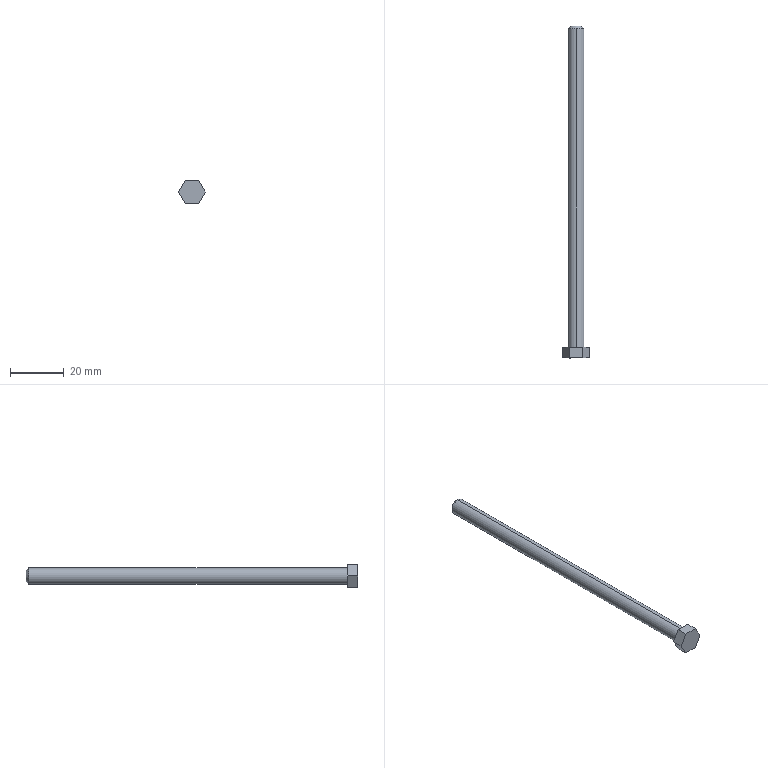Part | NX | features BREP 1 | 1 solid | 13 faces | box 10 x 124 x 8.66 mm | volume 3644 mm3 | plane 9 | cone 2 | cylinder 2 | commonest cylinder face diameters 6 x2
STEP:
#1=CARTESIAN_POINT('',(0.,124.,2.));
#2=VERTEX_POINT('',#1);
#3=CARTESIAN_POINT('',(0.,124.,-2.));
#4=VERTEX_POINT('',#3);
#5=CARTESIAN_POINT('',(0.,124.,0.));
#6=DIRECTION('',(0.,1.,0.));
#7=DIRECTION('',(0.,0.,1.));
#8=AXIS2_PLACEMENT_3D('',#5,#6,#7);
#9=CIRCLE('',#8,2.);
#10=EDGE_CURVE('',#2,#4,#9,.T.);
#11=ORIENTED_EDGE('',*,*,#10,.F.);
#12=CARTESIAN_POINT('',(0.,123.,3.));
#13=VERTEX_POINT('',#12);
#14=CARTESIAN_POINT('',(0.,124.,2.));
#15=DIRECTION('',(0.,-0.7071,0.7071));
#16=VECTOR('',#15,1000.);
#17=LINE('',#14,#16);
#18=EDGE_CURVE('',#13,#2,#17,.F.);
#19=ORIENTED_EDGE('',*,*,#18,.F.);
#20=CARTESIAN_POINT('',(0.,123.,-3.));
#21=VERTEX_POINT('',#20);
#22=CARTESIAN_POINT('',(0.,123.,0.));
#23=DIRECTION('',(0.,-1.,0.));
#24=DIRECTION('',(0.,0.,1.));
#25=AXIS2_PLACEMENT_3D('',#22,#23,#24);
#26=CIRCLE('',#25,3.);
#27=EDGE_CURVE('',#21,#13,#26,.T.);
#28=ORIENTED_EDGE('',*,*,#27,.F.);
#29=CARTESIAN_POINT('',(0.,124.,-2.));
#30=DIRECTION('',(0.,-0.7071,-0.7071));
#31=VECTOR('',#30,1000.);
#32=LINE('',#29,#31);
#33=EDGE_CURVE('',#21,#4,#32,.F.);
#34=ORIENTED_EDGE('',*,*,#33,.T.);
#35=EDGE_LOOP('',(#11,#19,#28,#34));
#36=FACE_BOUND('',#35,.T.);
#37=CARTESIAN_POINT('',(0.,124.,0.));
#38=DIRECTION('',(0.,-1.,0.));
#39=DIRECTION('',(0.,0.,1.));
#40=AXIS2_PLACEMENT_3D('',#37,#38,#39);
#41=CONICAL_SURFACE('',#40,2.,0.7854);
#42=ADVANCED_FACE('',(#36),#41,.T.);
#43=ORIENTED_EDGE('',*,*,#27,.T.);
#44=CARTESIAN_POINT('',(0.,4.,3.));
#45=VERTEX_POINT('',#44);
#46=CARTESIAN_POINT('',(0.,124.,3.));
#47=DIRECTION('',(0.,-1.,0.));
#48=VECTOR('',#47,1000.);
#49=LINE('',#46,#48);
#50=EDGE_CURVE('',#45,#13,#49,.F.);
#51=ORIENTED_EDGE('',*,*,#50,.F.);
#52=CARTESIAN_POINT('',(0.,4.,-3.));
#53=VERTEX_POINT('',#52);
#54=CARTESIAN_POINT('',(0.,4.,0.));
#55=DIRECTION('',(0.,1.,0.));
#56=DIRECTION('',(0.,0.,1.));
#57=AXIS2_PLACEMENT_3D('',#54,#55,#56);
#58=CIRCLE('',#57,3.);
#59=EDGE_CURVE('',#45,#53,#58,.T.);
#60=ORIENTED_EDGE('',*,*,#59,.T.);
#61=CARTESIAN_POINT('',(0.,124.,-3.));
#62=DIRECTION('',(0.,-1.,0.));
#63=VECTOR('',#62,1000.);
#64=LINE('',#61,#63);
#65=EDGE_CURVE('',#53,#21,#64,.F.);
#66=ORIENTED_EDGE('',*,*,#65,.T.);
#67=EDGE_LOOP('',(#43,#51,#60,#66));
#68=FACE_BOUND('',#67,.T.);
#69=CARTESIAN_POINT('',(0.,124.,0.));
#70=DIRECTION('',(0.,-1.,0.));
#71=DIRECTION('',(0.,0.,1.));
#72=AXIS2_PLACEMENT_3D('',#69,#70,#71);
#73=CYLINDRICAL_SURFACE('',#72,3.);
#74=ADVANCED_FACE('',(#68),#73,.T.);
#75=CARTESIAN_POINT('',(2.5,4.,4.33));
#76=VERTEX_POINT('',#75);
#77=CARTESIAN_POINT('',(5.,4.,0.));
#78=VERTEX_POINT('',#77);
#79=CARTESIAN_POINT('',(2.5,4.,4.33));
#80=DIRECTION('',(0.5,0.,-0.866));
#81=VECTOR('',#80,1000.);
#82=LINE('',#79,#81);
#83=EDGE_CURVE('',#76,#78,#82,.T.);
#84=ORIENTED_EDGE('',*,*,#83,.T.);
#85=CARTESIAN_POINT('',(2.5,4.,-4.33));
#86=VERTEX_POINT('',#85);
#87=CARTESIAN_POINT('',(5.,4.,0.));
#88=DIRECTION('',(-0.5,0.,-0.866));
#89=VECTOR('',#88,1000.);
#90=LINE('',#87,#89);
#91=EDGE_CURVE('',#78,#86,#90,.T.);
#92=ORIENTED_EDGE('',*,*,#91,.T.);
#93=CARTESIAN_POINT('',(-2.5,4.,-4.33));
#94=VERTEX_POINT('',#93);
#95=CARTESIAN_POINT('',(2.5,4.,-4.33));
#96=DIRECTION('',(-1.,0.,0.));
#97=VECTOR('',#96,1000.);
#98=LINE('',#95,#97);
#99=EDGE_CURVE('',#86,#94,#98,.T.);
#100=ORIENTED_EDGE('',*,*,#99,.T.);
#101=CARTESIAN_POINT('',(-5.,4.,0.));
#102=VERTEX_POINT('',#101);
#103=CARTESIAN_POINT('',(-2.5,4.,-4.33));
#104=DIRECTION('',(-0.5,0.,0.866));
#105=VECTOR('',#104,1000.);
#106=LINE('',#103,#105);
#107=EDGE_CURVE('',#94,#102,#106,.T.);
#108=ORIENTED_EDGE('',*,*,#107,.T.);
#109=CARTESIAN_POINT('',(-2.5,4.,4.33));
#110=VERTEX_POINT('',#109);
#111=CARTESIAN_POINT('',(-5.,4.,0.));
#112=DIRECTION('',(0.5,0.,0.866));
#113=VECTOR('',#112,1000.);
#114=LINE('',#111,#113);
#115=EDGE_CURVE('',#102,#110,#114,.T.);
#116=ORIENTED_EDGE('',*,*,#115,.T.);
#117=CARTESIAN_POINT('',(-2.5,4.,4.33));
#118=DIRECTION('',(1.,0.,0.));
#119=VECTOR('',#118,1000.);
#120=LINE('',#117,#119);
#121=EDGE_CURVE('',#110,#76,#120,.T.);
#122=ORIENTED_EDGE('',*,*,#121,.T.);
#123=EDGE_LOOP('',(#84,#92,#100,#108,#116,#122));
#124=FACE_BOUND('',#123,.T.);
#125=CARTESIAN_POINT('',(0.,4.,0.));
#126=DIRECTION('',(0.,1.,0.));
#127=DIRECTION('',(0.,0.,1.));
#128=AXIS2_PLACEMENT_3D('',#125,#126,#127);
#129=CIRCLE('',#128,3.);
#130=EDGE_CURVE('',#53,#45,#129,.T.);
#131=ORIENTED_EDGE('',*,*,#130,.F.);
#132=ORIENTED_EDGE('',*,*,#59,.F.);
#133=EDGE_LOOP('',(#131,#132));
#134=FACE_BOUND('',#133,.T.);
#135=CARTESIAN_POINT('',(0.,4.,0.));
#136=DIRECTION('',(0.,1.,0.));
#137=DIRECTION('',(0.,0.,1.));
#138=AXIS2_PLACEMENT_3D('',#135,#136,#137);
#139=PLANE('',#138);
#140=ADVANCED_FACE('',(#124,#134),#139,.T.);
#141=CARTESIAN_POINT('',(2.5,0.,4.33));
#142=VERTEX_POINT('',#141);
#143=CARTESIAN_POINT('',(5.,0.,0.));
#144=VERTEX_POINT('',#143);
#145=CARTESIAN_POINT('',(2.5,0.,4.33));
#146=DIRECTION('',(0.5,0.,-0.866));
#147=VECTOR('',#146,1000.);
#148=LINE('',#145,#147);
#149=EDGE_CURVE('',#142,#144,#148,.T.);
#150=ORIENTED_EDGE('',*,*,#149,.T.);
#151=CARTESIAN_POINT('',(5.,4.,0.));
#152=DIRECTION('',(0.,-1.,0.));
#153=VECTOR('',#152,1000.);
#154=LINE('',#151,#153);
#155=EDGE_CURVE('',#78,#144,#154,.T.);
#156=ORIENTED_EDGE('',*,*,#155,.F.);
#157=ORIENTED_EDGE('',*,*,#83,.F.);
#158=CARTESIAN_POINT('',(2.5,4.,4.33));
#159=DIRECTION('',(0.,-1.,0.));
#160=VECTOR('',#159,1000.);
#161=LINE('',#158,#160);
#162=EDGE_CURVE('',#76,#142,#161,.T.);
#163=ORIENTED_EDGE('',*,*,#162,.T.);
#164=EDGE_LOOP('',(#150,#156,#157,#163));
#165=FACE_BOUND('',#164,.T.);
#166=CARTESIAN_POINT('',(2.5,4.,4.33));
#167=DIRECTION('',(-0.866,0.,-0.5));
#168=DIRECTION('',(0.5,0.,-0.866));
#169=AXIS2_PLACEMENT_3D('',#166,#167,#168);
#170=PLANE('',#169);
#171=ADVANCED_FACE('',(#165),#170,.F.);
#172=CARTESIAN_POINT('',(2.5,0.,-4.33));
#173=VERTEX_POINT('',#172);
#174=CARTESIAN_POINT('',(5.,0.,0.));
#175=DIRECTION('',(-0.5,0.,-0.866));
#176=VECTOR('',#175,1000.);
#177=LINE('',#174,#176);
#178=EDGE_CURVE('',#144,#173,#177,.T.);
#179=ORIENTED_EDGE('',*,*,#178,.T.);
#180=CARTESIAN_POINT('',(2.5,4.,-4.33));
#181=DIRECTION('',(0.,-1.,0.));
#182=VECTOR('',#181,1000.);
#183=LINE('',#180,#182);
#184=EDGE_CURVE('',#86,#173,#183,.T.);
#185=ORIENTED_EDGE('',*,*,#184,.F.);
#186=ORIENTED_EDGE('',*,*,#91,.F.);
#187=ORIENTED_EDGE('',*,*,#155,.T.);
#188=EDGE_LOOP('',(#179,#185,#186,#187));
#189=FACE_BOUND('',#188,.T.);
#190=CARTESIAN_POINT('',(5.,4.,0.));
#191=DIRECTION('',(-0.866,0.,0.5));
#192=DIRECTION('',(0.,-1.,0.));
#193=AXIS2_PLACEMENT_3D('',#190,#191,#192);
#194=PLANE('',#193);
#195=ADVANCED_FACE('',(#189),#194,.F.);
#196=CARTESIAN_POINT('',(-2.5,0.,-4.33));
#197=VERTEX_POINT('',#196);
#198=CARTESIAN_POINT('',(2.5,0.,-4.33));
#199=DIRECTION('',(-1.,0.,0.));
#200=VECTOR('',#199,1000.);
#201=LINE('',#198,#200);
#202=EDGE_CURVE('',#173,#197,#201,.T.);
#203=ORIENTED_EDGE('',*,*,#202,.T.);
#204=CARTESIAN_POINT('',(-2.5,4.,-4.33));
#205=DIRECTION('',(0.,-1.,0.));
#206=VECTOR('',#205,1000.);
#207=LINE('',#204,#206);
#208=EDGE_CURVE('',#94,#197,#207,.T.);
#209=ORIENTED_EDGE('',*,*,#208,.F.);
#210=ORIENTED_EDGE('',*,*,#99,.F.);
#211=ORIENTED_EDGE('',*,*,#184,.T.);
#212=EDGE_LOOP('',(#203,#209,#210,#211));
#213=FACE_BOUND('',#212,.T.);
#214=CARTESIAN_POINT('',(2.5,4.,-4.33));
#215=DIRECTION('',(0.,0.,1.));
#216=DIRECTION('',(-1.,0.,0.));
#217=AXIS2_PLACEMENT_3D('',#214,#215,#216);
#218=PLANE('',#217);
#219=ADVANCED_FACE('',(#213),#218,.F.);
#220=CARTESIAN_POINT('',(-5.,0.,0.));
#221=VERTEX_POINT('',#220);
#222=CARTESIAN_POINT('',(-2.5,0.,-4.33));
#223=DIRECTION('',(-0.5,0.,0.866));
#224=VECTOR('',#223,1000.);
#225=LINE('',#222,#224);
#226=EDGE_CURVE('',#197,#221,#225,.T.);
#227=ORIENTED_EDGE('',*,*,#226,.T.);
#228=CARTESIAN_POINT('',(-5.,4.,0.));
#229=DIRECTION('',(0.,-1.,0.));
#230=VECTOR('',#229,1000.);
#231=LINE('',#228,#230);
#232=EDGE_CURVE('',#102,#221,#231,.T.);
#233=ORIENTED_EDGE('',*,*,#232,.F.);
#234=ORIENTED_EDGE('',*,*,#107,.F.);
#235=ORIENTED_EDGE('',*,*,#208,.T.);
#236=EDGE_LOOP('',(#227,#233,#234,#235));
#237=FACE_BOUND('',#236,.T.);
#238=CARTESIAN_POINT('',(-2.5,4.,-4.33));
#239=DIRECTION('',(0.866,0.,0.5));
#240=DIRECTION('',(0.,1.,0.));
#241=AXIS2_PLACEMENT_3D('',#238,#239,#240);
#242=PLANE('',#241);
#243=ADVANCED_FACE('',(#237),#242,.F.);
#244=CARTESIAN_POINT('',(-2.5,0.,4.33));
#245=VERTEX_POINT('',#244);
#246=CARTESIAN_POINT('',(-5.,0.,0.));
#247=DIRECTION('',(0.5,0.,0.866));
#248=VECTOR('',#247,1000.);
#249=LINE('',#246,#248);
#250=EDGE_CURVE('',#221,#245,#249,.T.);
#251=ORIENTED_EDGE('',*,*,#250,.T.);
#252=CARTESIAN_POINT('',(-2.5,4.,4.33));
#253=DIRECTION('',(0.,-1.,0.));
#254=VECTOR('',#253,1000.);
#255=LINE('',#252,#254);
#256=EDGE_CURVE('',#110,#245,#255,.T.);
#257=ORIENTED_EDGE('',*,*,#256,.F.);
#258=ORIENTED_EDGE('',*,*,#115,.F.);
#259=ORIENTED_EDGE('',*,*,#232,.T.);
#260=EDGE_LOOP('',(#251,#257,#258,#259));
#261=FACE_BOUND('',#260,.T.);
#262=CARTESIAN_POINT('',(-5.,4.,0.));
#263=DIRECTION('',(0.866,0.,-0.5));
#264=DIRECTION('',(0.,1.,0.));
#265=AXIS2_PLACEMENT_3D('',#262,#263,#264);
#266=PLANE('',#265);
#267=ADVANCED_FACE('',(#261),#266,.F.);
#268=CARTESIAN_POINT('',(-2.5,0.,4.33));
#269=DIRECTION('',(1.,0.,0.));
#270=VECTOR('',#269,1000.);
#271=LINE('',#268,#270);
#272=EDGE_CURVE('',#245,#142,#271,.T.);
#273=ORIENTED_EDGE('',*,*,#272,.T.);
#274=ORIENTED_EDGE('',*,*,#162,.F.);
#275=ORIENTED_EDGE('',*,*,#121,.F.);
#276=ORIENTED_EDGE('',*,*,#256,.T.);
#277=EDGE_LOOP('',(#273,#274,#275,#276));
#278=FACE_BOUND('',#277,.T.);
#279=CARTESIAN_POINT('',(-2.5,4.,4.33));
#280=DIRECTION('',(0.,0.,-1.));
#281=DIRECTION('',(1.,0.,0.));
#282=AXIS2_PLACEMENT_3D('',#279,#280,#281);
#283=PLANE('',#282);
#284=ADVANCED_FACE('',(#278),#283,.F.);
#285=ORIENTED_EDGE('',*,*,#149,.F.);
#286=ORIENTED_EDGE('',*,*,#272,.F.);
#287=ORIENTED_EDGE('',*,*,#250,.F.);
#288=ORIENTED_EDGE('',*,*,#226,.F.);
#289=ORIENTED_EDGE('',*,*,#202,.F.);
#290=ORIENTED_EDGE('',*,*,#178,.F.);
#291=EDGE_LOOP('',(#285,#286,#287,#288,#289,#290));
#292=FACE_BOUND('',#291,.T.);
#293=CARTESIAN_POINT('',(0.,0.,0.));
#294=DIRECTION('',(0.,1.,0.));
#295=DIRECTION('',(0.,0.,1.));
#296=AXIS2_PLACEMENT_3D('',#293,#294,#295);
#297=PLANE('',#296);
#298=ADVANCED_FACE('',(#292),#297,.F.);
#299=ORIENTED_EDGE('',*,*,#50,.T.);
#300=CARTESIAN_POINT('',(0.,123.,0.));
#301=DIRECTION('',(0.,-1.,0.));
#302=DIRECTION('',(0.,0.,1.));
#303=AXIS2_PLACEMENT_3D('',#300,#301,#302);
#304=CIRCLE('',#303,3.);
#305=EDGE_CURVE('',#13,#21,#304,.T.);
#306=ORIENTED_EDGE('',*,*,#305,.T.);
#307=ORIENTED_EDGE('',*,*,#65,.F.);
#308=ORIENTED_EDGE('',*,*,#130,.T.);
#309=EDGE_LOOP('',(#299,#306,#307,#308));
#310=FACE_BOUND('',#309,.T.);
#311=CARTESIAN_POINT('',(0.,124.,0.));
#312=DIRECTION('',(0.,-1.,0.));
#313=DIRECTION('',(0.,0.,1.));
#314=AXIS2_PLACEMENT_3D('',#311,#312,#313);
#315=CYLINDRICAL_SURFACE('',#314,3.);
#316=ADVANCED_FACE('',(#310),#315,.T.);
#317=CARTESIAN_POINT('',(0.,124.,0.));
#318=DIRECTION('',(0.,1.,0.));
#319=DIRECTION('',(0.,0.,1.));
#320=AXIS2_PLACEMENT_3D('',#317,#318,#319);
#321=CIRCLE('',#320,2.);
#322=EDGE_CURVE('',#4,#2,#321,.T.);
#323=ORIENTED_EDGE('',*,*,#322,.T.);
#324=ORIENTED_EDGE('',*,*,#10,.T.);
#325=EDGE_LOOP('',(#323,#324));
#326=FACE_BOUND('',#325,.T.);
#327=CARTESIAN_POINT('',(0.,124.,0.));
#328=DIRECTION('',(0.,1.,0.));
#329=DIRECTION('',(0.,0.,1.));
#330=AXIS2_PLACEMENT_3D('',#327,#328,#329);
#331=PLANE('',#330);
#332=ADVANCED_FACE('',(#326),#331,.T.);
#333=ORIENTED_EDGE('',*,*,#18,.T.);
#334=ORIENTED_EDGE('',*,*,#322,.F.);
#335=ORIENTED_EDGE('',*,*,#33,.F.);
#336=ORIENTED_EDGE('',*,*,#305,.F.);
#337=EDGE_LOOP('',(#333,#334,#335,#336));
#338=FACE_BOUND('',#337,.T.);
#339=CARTESIAN_POINT('',(0.,124.,0.));
#340=DIRECTION('',(0.,-1.,0.));
#341=DIRECTION('',(0.,0.,1.));
#342=AXIS2_PLACEMENT_3D('',#339,#340,#341);
#343=CONICAL_SURFACE('',#342,2.,0.7854);
#344=ADVANCED_FACE('',(#338),#343,.T.);
#345=CLOSED_SHELL('',(#42,#74,#140,#171,#195,#219,#243,#267,#284,#298,#316,#332,#344));
#346=MANIFOLD_SOLID_BREP('',#345);
#347=(LENGTH_UNIT()NAMED_UNIT(*)SI_UNIT(.MILLI.,.METRE.));
#348=UNCERTAINTY_MEASURE_WITH_UNIT(LENGTH_MEASURE(0.00001),#347,'','');
#349=(NAMED_UNIT(*)PLANE_ANGLE_UNIT()SI_UNIT($,.RADIAN.));
#350=(NAMED_UNIT(*)SI_UNIT($,.STERADIAN.)SOLID_ANGLE_UNIT());
#351=(GEOMETRIC_REPRESENTATION_CONTEXT(3)GLOBAL_UNCERTAINTY_ASSIGNED_CONTEXT((#348))GLOBAL_UNIT_ASSIGNED_CONTEXT((#347,#349,#350))REPRESENTATION_CONTEXT('',''));
#352=ADVANCED_BREP_SHAPE_REPRESENTATION('',(#346),#351);